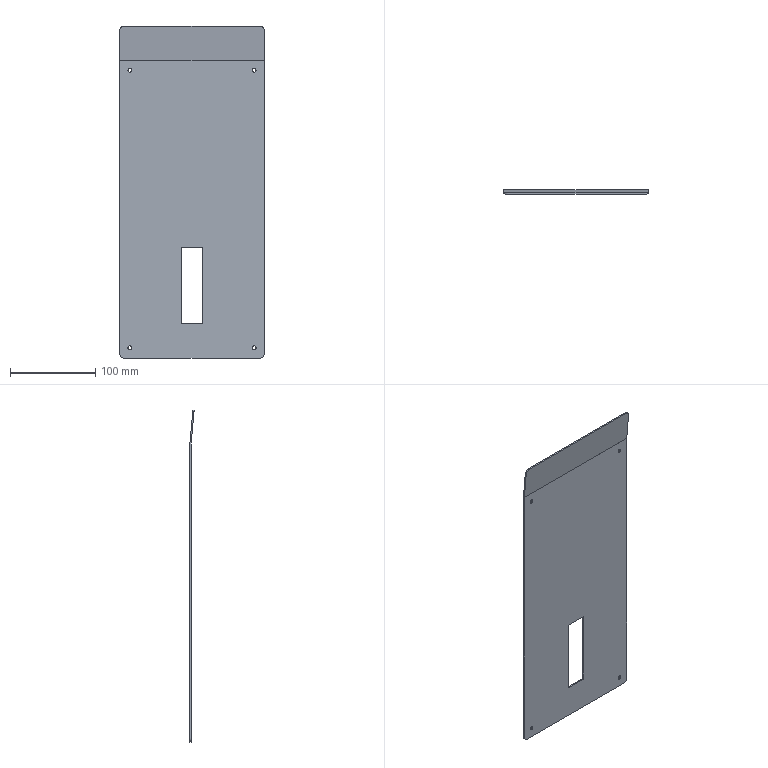Part | STEP file | B1-021 | 1 solid | 30 faces | box 170 x 4.986 x 389.979 mm | volume 95964 mm3 | plane 16 | cylinder 14 | commonest cylinder face diameters 4.5 x8 10 x4 1 x1 4 x1